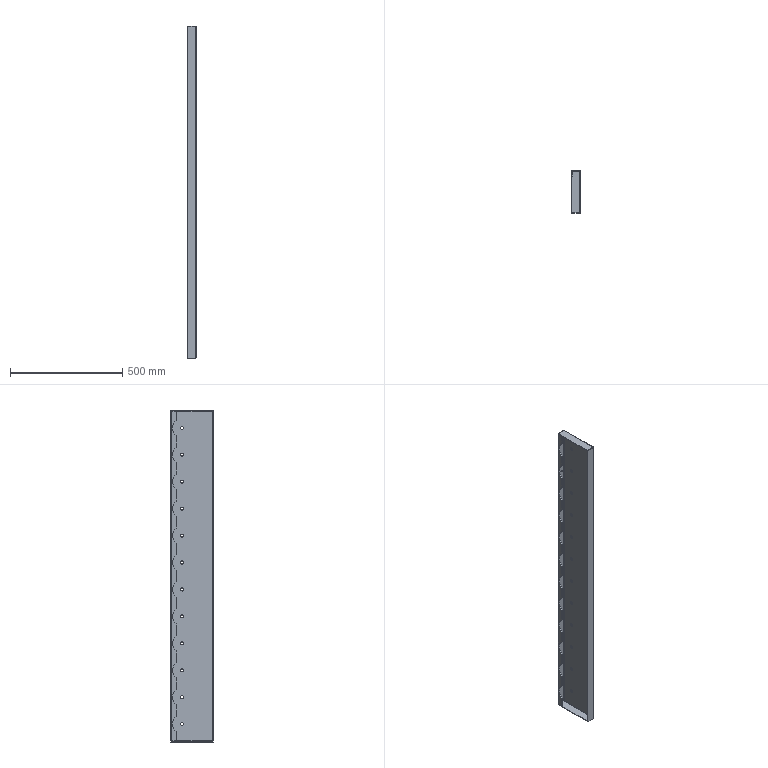Part | STEP file | 8-Body driven side | 1 solid | 148 faces | box 40 x 189 x 1480 mm | volume 1252545 mm3 | plane 82 | cylinder 66 | commonest cylinder face diameters 11 x36 84 x12 6.8 x8 3 x5 9 x5